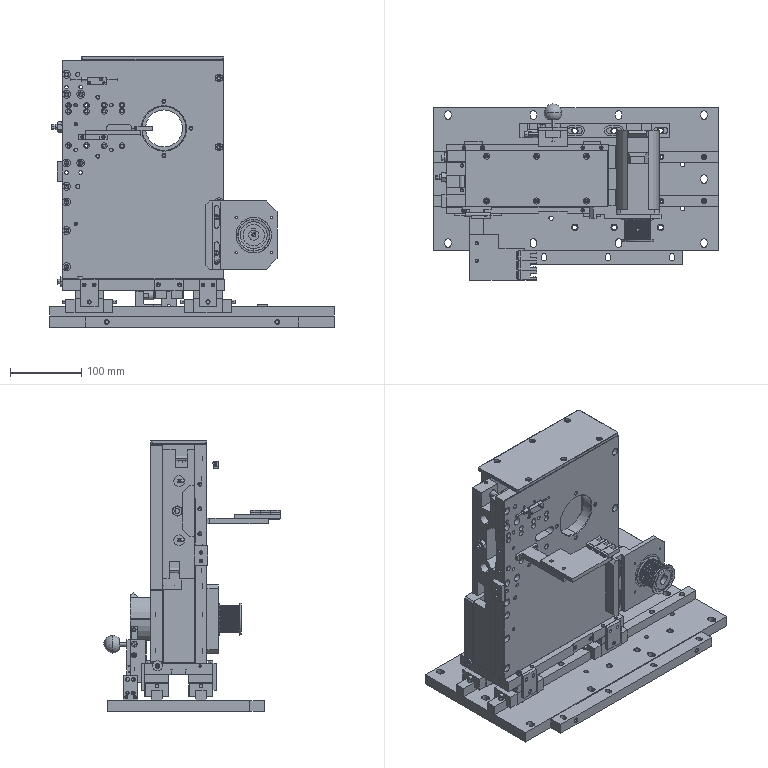Part | NX | 67 solids | 4063 faces | volume 5170409 mm3 | plane 2038 | cylinder 1435 | cone 538 | spline 44 | sphere 8 | commonest cylinder face diameters 5 x403 3.3 x144 0.5 x52 4.5 x52 6.55 x52 1.1 x48